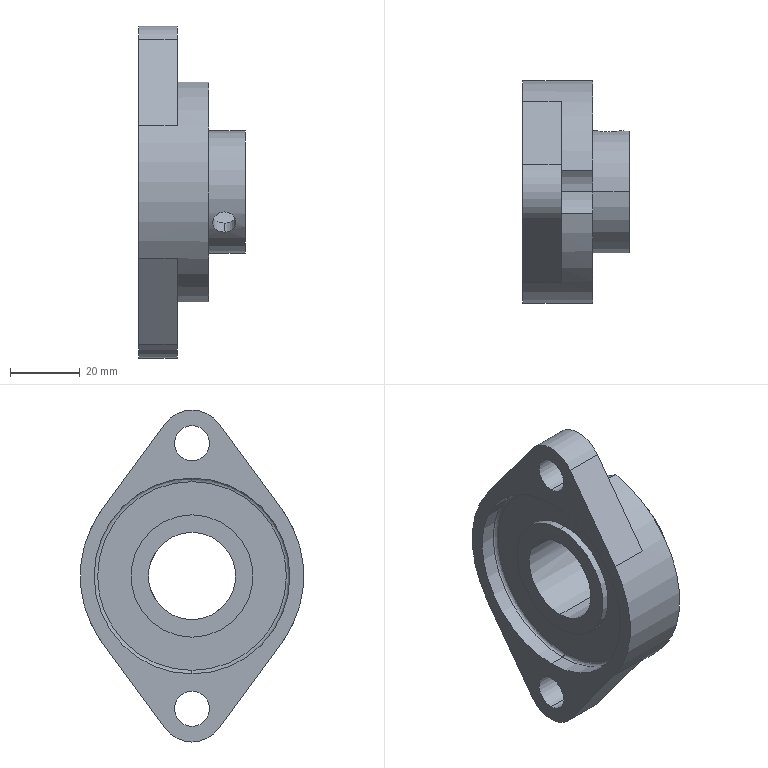Part | SolidWorks | features BaseBody 1 | 1 solid | 42 faces | box 30.5 x 64 x 95 mm | volume 50560 mm3 | cylinder 26 | plane 12 | spline 4 | commonest cylinder face diameters 6.647 x4 10 x4 35 x4 56 x4 18 x3 19 x3